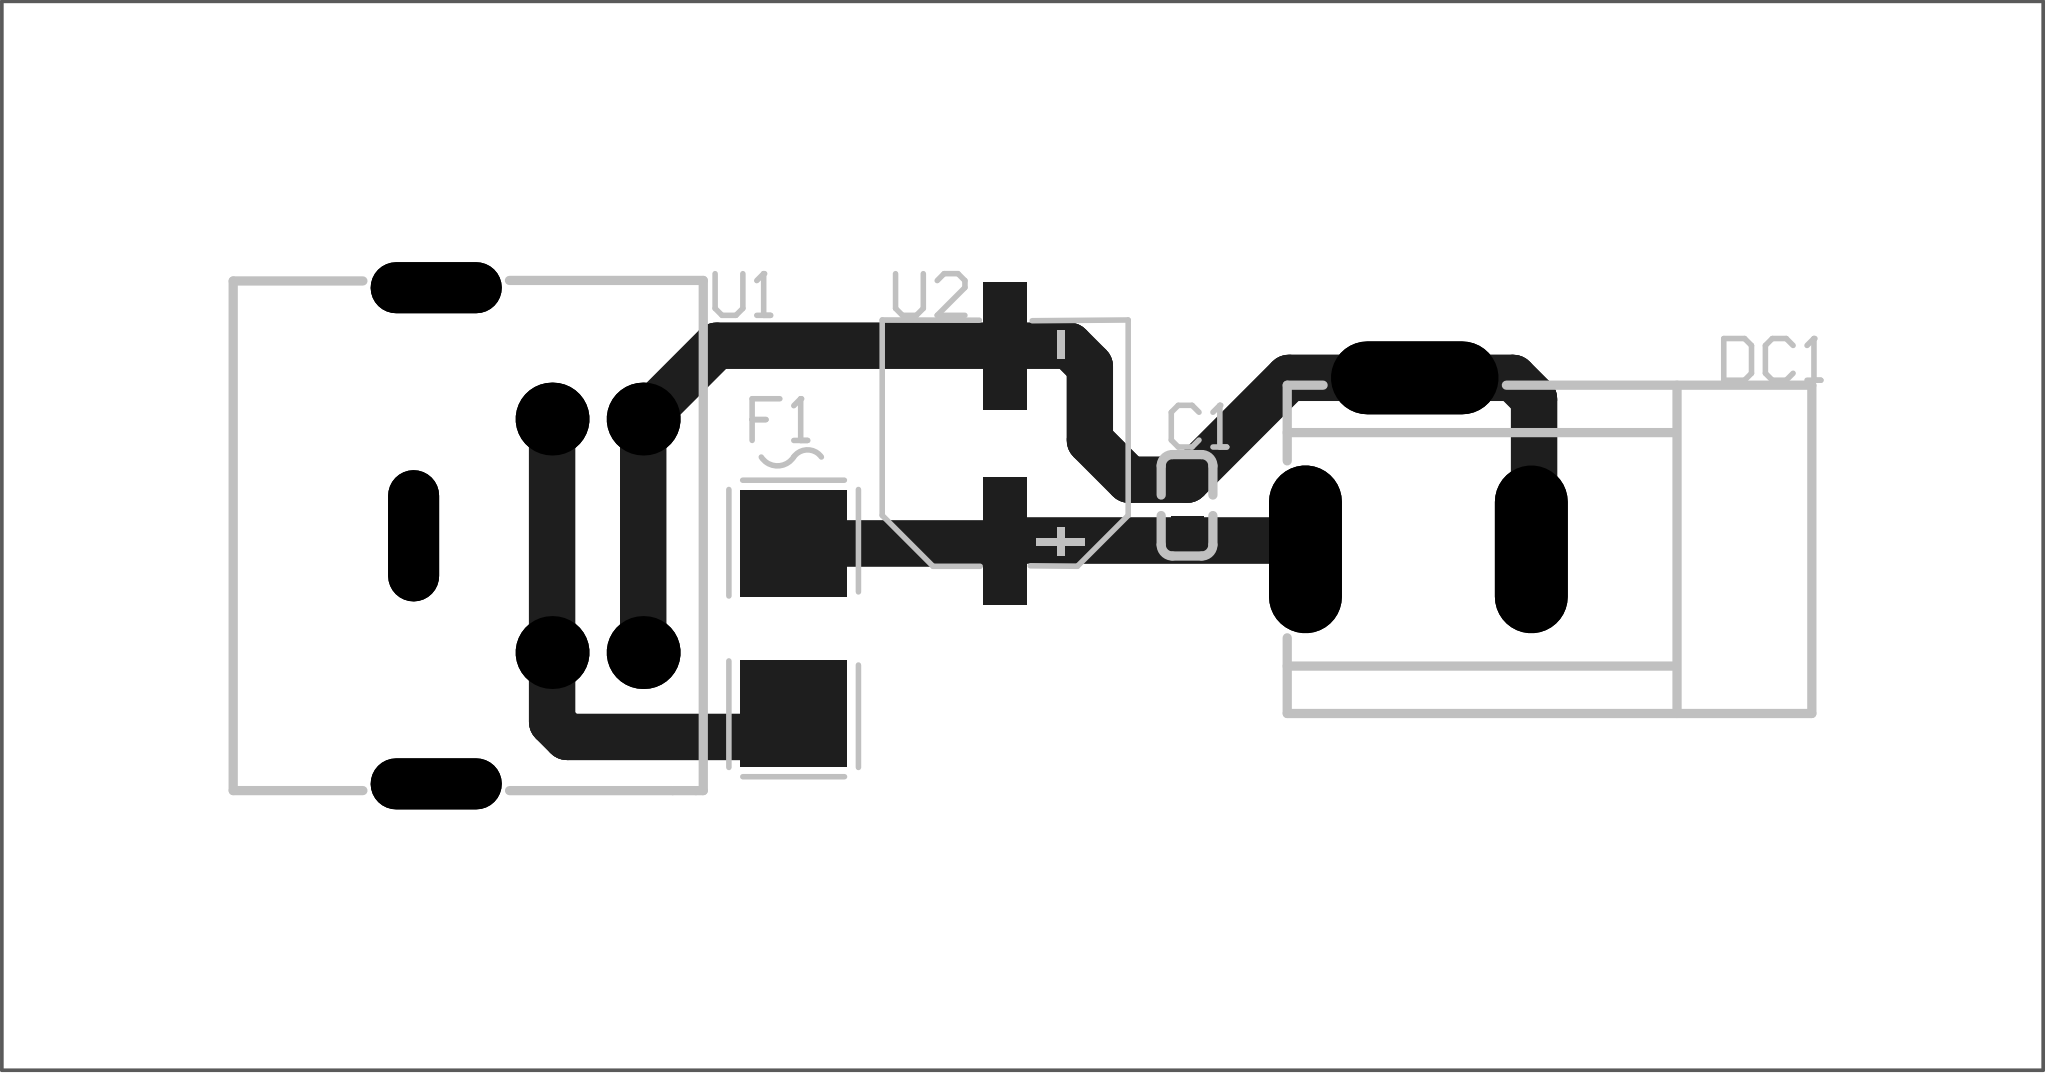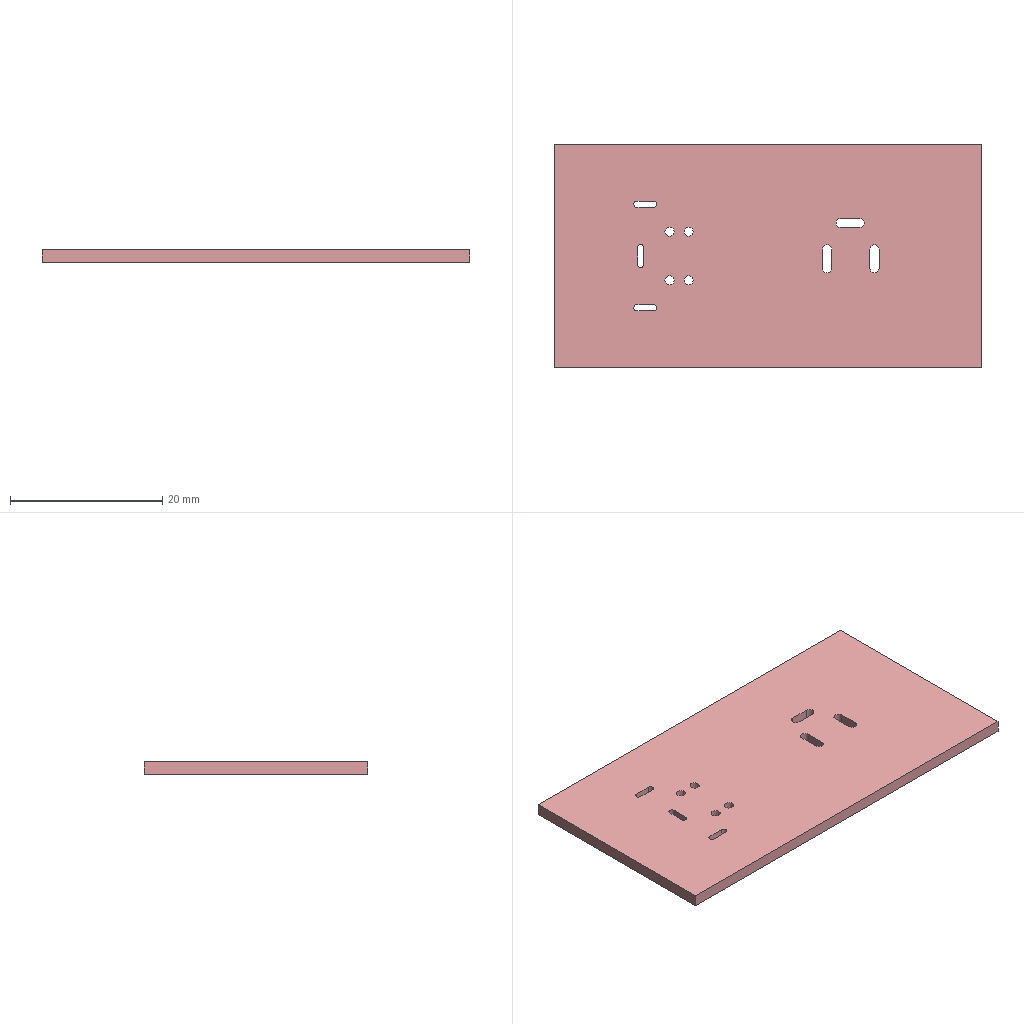Circuit board layout | Altium Designer | box 56 x 29.3 x 1.6 mm
Layer stack:
# Altium Designer layer stack of  (unit mm; dielectric type: 0 none, 1 core, 2 prepreg, 3 surface material)
index,name,kind,layer,copper_thickness_mm,dielectric_type,dielectric_thickness_mm,dielectric_material,dielectric_constant
0,Top Paste Mask Layer,other,,,,,,
1,Top Silkscreen Layer,other,,,,,,
2,Top Solder Mask Layer,dielectric,,,3,0.01,,3.3
3,Top Layer,copper,Top Layer,0.035,,,,
4,Dielectric1,dielectric,,,3,1.51,FR4,4.5
5,Bottom Layer,copper,Bottom Layer,0.035,,,,
6,Bottom Solder Mask Layer,dielectric,,,3,0.01,,3.3
7,Bottom Silkscreen Layer,other,,,,,,
8,Bottom Paste Mask Layer,other,,,,,,
# drill layer pairs: low layer,high layer
drill_pair,Top Layer,Bottom Layer
Part placement:
Designator,Comment,Layer,Footprint,Center-X(mm),Center-Y(mm),Rotation
C1,10uF,TopLayer,C0603,102.382,85.336,90
DC1,DC005,TopLayer,DC-IN-TH_DC005,108.732,86.479,180
F1,10A保险丝,TopLayer,FUSE-SMD_L6.1-W2.6,91.584,81.96,270
U1,M-DIN_4-R母座,TopLayer,CONN-TH_DIN_4P_12D8,84.303,84.5,90
U2,100uF贴片电解,TopLayer,CAP-SMD_BD6.3-L6.6-W6.6-LS7.4-FD,97.391,87.04,90
Pad and via stacks:
# Altium Designer via and pad stacks of  (unit mm). Each distinct definition once, with the count of objects using it.
# via: kind,start_layer,end_layer,hole_mm,diameter_mm,mode(0 simple;1 top-mid-bottom;2 full stack),diameter_per_layer,count,example_net
# pad: kind,layer,hole_mm,hole_type(0 round;1 square;2 slot),plating,top_size,top_shape(1 round;2 rect;3 octagon;9 rounded rect),mid_size,bottom_size,mode,footprint,size_per_layer,count,example
pad,Top Layer,0,0,plated,0.8x0.9,2,0.8x0.9,0.8x0.9,0,C0603,,2,C1.2
pad,Top Layer,0,0,plated,2.91x2.911,2,2.91x2.911,2.91x2.911,0,FUSE-SMD_L6.1-W2.6,,2,F1.2
pad,Top Layer,0,0,plated,3.5x1.2,2,3.5x1.2,3.5x1.2,0,CAP-SMD_BD6.3-L6.6-W6.6-LS7.4-FD,,2,U2.1
pad,Multi-Layer,1.2,2,plated,2x4.6,1,2x4.6,2x4.6,0,DC-IN-TH_DC005,,2,DC1.1
pad,Multi-Layer,1.2,2,plated,4.6x2,1,4.6x2,4.6x2,0,DC-IN-TH_DC005,,1,DC1.3
pad,Multi-Layer,1.2,0,plated,2x2,1,2x2,2x2,0,CONN-TH_DIN_4P_12D8,,4,U1.1
pad,Multi-Layer,0.8,2,plated,3.6x1.4,1,3.6x1.4,3.6x1.4,0,CONN-TH_DIN_4P_12D8,,1,U1.5
pad,Multi-Layer,0.8,2,plated,1.4x3.6,1,1.4x3.6,1.4x3.6,0,CONN-TH_DIN_4P_12D8,,2,U1.6